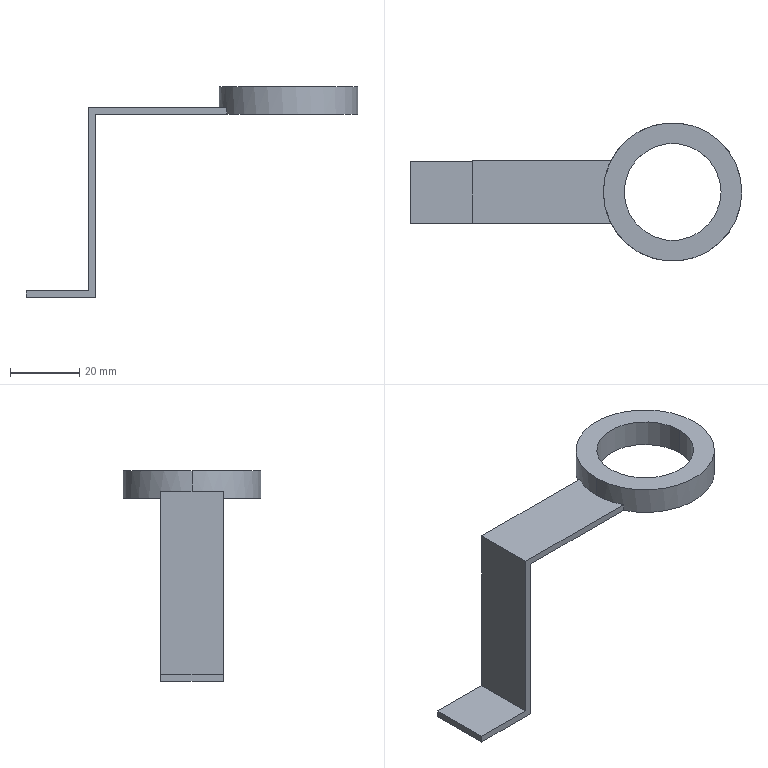Part | SolidWorks | features ICE 3, Extrusion 1 | 1 solid | 14 faces | box 95.861 x 40 x 61 mm | volume 9071 mm3 | plane 10 | cylinder 4 | commonest cylinder face diameters 28 x2 40 x2
STEP:
#1=CARTESIAN_POINT('',(-14.,0.,4.));
#2=VERTEX_POINT('',#1);
#3=CARTESIAN_POINT('',(14.,0.,4.));
#4=VERTEX_POINT('',#3);
#5=CARTESIAN_POINT('',(0.,0.,4.));
#6=DIRECTION('',(0.,0.,1.));
#7=DIRECTION('',(1.,0.,0.));
#8=AXIS2_PLACEMENT_3D('',#5,#6,#7);
#9=CIRCLE('',#8,14.);
#10=EDGE_CURVE('',#2,#4,#9,.T.);
#11=ORIENTED_EDGE('',*,*,#10,.T.);
#12=CARTESIAN_POINT('',(14.,0.,-4.));
#13=VERTEX_POINT('',#12);
#14=CARTESIAN_POINT('',(14.,0.,4.));
#15=DIRECTION('',(0.,0.,-1.));
#16=VECTOR('',#15,1000.);
#17=LINE('',#14,#16);
#18=EDGE_CURVE('',#4,#13,#17,.T.);
#19=ORIENTED_EDGE('',*,*,#18,.T.);
#20=CARTESIAN_POINT('',(-14.,0.,-4.));
#21=VERTEX_POINT('',#20);
#22=CARTESIAN_POINT('',(0.,0.,-4.));
#23=DIRECTION('',(0.,0.,1.));
#24=DIRECTION('',(1.,0.,0.));
#25=AXIS2_PLACEMENT_3D('',#22,#23,#24);
#26=CIRCLE('',#25,14.);
#27=EDGE_CURVE('',#21,#13,#26,.T.);
#28=ORIENTED_EDGE('',*,*,#27,.F.);
#29=CARTESIAN_POINT('',(-14.,0.,4.));
#30=DIRECTION('',(0.,0.,-1.));
#31=VECTOR('',#30,1000.);
#32=LINE('',#29,#31);
#33=EDGE_CURVE('',#2,#21,#32,.T.);
#34=ORIENTED_EDGE('',*,*,#33,.F.);
#35=EDGE_LOOP('',(#11,#19,#28,#34));
#36=FACE_OUTER_BOUND('',#35,.T.);
#37=CARTESIAN_POINT('',(0.,0.,4.));
#38=DIRECTION('',(0.,0.,-1.));
#39=DIRECTION('',(-1.,0.,0.));
#40=AXIS2_PLACEMENT_3D('',#37,#38,#39);
#41=CYLINDRICAL_SURFACE('',#40,14.);
#42=ADVANCED_FACE('',(#36),#41,.F.);
#43=CARTESIAN_POINT('',(20.,0.,4.));
#44=VERTEX_POINT('',#43);
#45=CARTESIAN_POINT('',(-20.,0.,4.));
#46=VERTEX_POINT('',#45);
#47=CARTESIAN_POINT('',(0.,0.,4.));
#48=DIRECTION('',(0.,0.,1.));
#49=DIRECTION('',(1.,0.,0.));
#50=AXIS2_PLACEMENT_3D('',#47,#48,#49);
#51=CIRCLE('',#50,20.);
#52=EDGE_CURVE('',#44,#46,#51,.T.);
#53=ORIENTED_EDGE('',*,*,#52,.F.);
#54=CARTESIAN_POINT('',(20.,0.,-4.));
#55=VERTEX_POINT('',#54);
#56=CARTESIAN_POINT('',(20.,0.,4.));
#57=DIRECTION('',(0.,0.,-1.));
#58=VECTOR('',#57,1000.);
#59=LINE('',#56,#58);
#60=EDGE_CURVE('',#44,#55,#59,.T.);
#61=ORIENTED_EDGE('',*,*,#60,.T.);
#62=CARTESIAN_POINT('',(-17.861,9.,-4.));
#63=VERTEX_POINT('',#62);
#64=CARTESIAN_POINT('',(0.,0.,-4.));
#65=DIRECTION('',(0.,0.,1.));
#66=DIRECTION('',(1.,0.,0.));
#67=AXIS2_PLACEMENT_3D('',#64,#65,#66);
#68=CIRCLE('',#67,20.);
#69=EDGE_CURVE('',#55,#63,#68,.T.);
#70=ORIENTED_EDGE('',*,*,#69,.T.);
#71=CARTESIAN_POINT('',(-17.861,9.,-2.));
#72=VERTEX_POINT('',#71);
#73=CARTESIAN_POINT('',(-17.861,9.,-2.));
#74=DIRECTION('',(0.,0.,-1.));
#75=VECTOR('',#74,1000.);
#76=LINE('',#73,#75);
#77=EDGE_CURVE('',#72,#63,#76,.T.);
#78=ORIENTED_EDGE('',*,*,#77,.F.);
#79=CARTESIAN_POINT('',(-20.,0.,-2.));
#80=VERTEX_POINT('',#79);
#81=CARTESIAN_POINT('',(0.,0.,-2.));
#82=DIRECTION('',(0.,0.,1.));
#83=DIRECTION('',(1.,0.,0.));
#84=AXIS2_PLACEMENT_3D('',#81,#82,#83);
#85=CIRCLE('',#84,20.);
#86=EDGE_CURVE('',#72,#80,#85,.T.);
#87=ORIENTED_EDGE('',*,*,#86,.T.);
#88=CARTESIAN_POINT('',(-20.,0.,4.));
#89=DIRECTION('',(0.,0.,-1.));
#90=VECTOR('',#89,1000.);
#91=LINE('',#88,#90);
#92=EDGE_CURVE('',#46,#80,#91,.T.);
#93=ORIENTED_EDGE('',*,*,#92,.F.);
#94=EDGE_LOOP('',(#53,#61,#70,#78,#87,#93));
#95=FACE_OUTER_BOUND('',#94,.T.);
#96=CARTESIAN_POINT('',(0.,0.,4.));
#97=DIRECTION('',(0.,0.,-1.));
#98=DIRECTION('',(-1.,0.,0.));
#99=AXIS2_PLACEMENT_3D('',#96,#97,#98);
#100=CYLINDRICAL_SURFACE('',#99,20.);
#101=ADVANCED_FACE('',(#95),#100,.T.);
#102=ORIENTED_EDGE('',*,*,#27,.T.);
#103=CARTESIAN_POINT('',(0.,0.,-4.));
#104=DIRECTION('',(0.,0.,1.));
#105=DIRECTION('',(1.,0.,0.));
#106=AXIS2_PLACEMENT_3D('',#103,#104,#105);
#107=CIRCLE('',#106,14.);
#108=EDGE_CURVE('',#13,#21,#107,.T.);
#109=ORIENTED_EDGE('',*,*,#108,.T.);
#110=EDGE_LOOP('',(#102,#109));
#111=FACE_BOUND('',#110,.T.);
#112=CARTESIAN_POINT('',(-55.861,9.,-4.));
#113=VERTEX_POINT('',#112);
#114=CARTESIAN_POINT('',(-55.861,-9.,-4.));
#115=VERTEX_POINT('',#114);
#116=CARTESIAN_POINT('',(-55.861,9.,-4.));
#117=DIRECTION('',(0.,-1.,0.));
#118=VECTOR('',#117,1000.);
#119=LINE('',#116,#118);
#120=EDGE_CURVE('',#113,#115,#119,.T.);
#121=ORIENTED_EDGE('',*,*,#120,.F.);
#122=CARTESIAN_POINT('',(-17.861,9.,-4.));
#123=DIRECTION('',(1.,0.,0.));
#124=VECTOR('',#123,1000.);
#125=LINE('',#122,#124);
#126=EDGE_CURVE('',#113,#63,#125,.T.);
#127=ORIENTED_EDGE('',*,*,#126,.T.);
#128=ORIENTED_EDGE('',*,*,#69,.F.);
#129=CARTESIAN_POINT('',(-17.861,-9.,-4.));
#130=VERTEX_POINT('',#129);
#131=CARTESIAN_POINT('',(0.,0.,-4.));
#132=DIRECTION('',(0.,0.,1.));
#133=DIRECTION('',(1.,0.,0.));
#134=AXIS2_PLACEMENT_3D('',#131,#132,#133);
#135=CIRCLE('',#134,20.);
#136=EDGE_CURVE('',#130,#55,#135,.T.);
#137=ORIENTED_EDGE('',*,*,#136,.F.);
#138=CARTESIAN_POINT('',(-57.861,-9.,-4.));
#139=DIRECTION('',(-1.,0.,0.));
#140=VECTOR('',#139,1000.);
#141=LINE('',#138,#140);
#142=EDGE_CURVE('',#130,#115,#141,.T.);
#143=ORIENTED_EDGE('',*,*,#142,.T.);
#144=EDGE_LOOP('',(#121,#127,#128,#137,#143));
#145=FACE_OUTER_BOUND('',#144,.T.);
#146=CARTESIAN_POINT('',(0.,0.,-4.));
#147=DIRECTION('',(0.,0.,1.));
#148=DIRECTION('',(1.,0.,0.));
#149=AXIS2_PLACEMENT_3D('',#146,#147,#148);
#150=PLANE('',#149);
#151=ADVANCED_FACE('',(#111,#145),#150,.F.);
#152=CARTESIAN_POINT('',(0.,0.,4.));
#153=DIRECTION('',(0.,0.,1.));
#154=DIRECTION('',(1.,0.,0.));
#155=AXIS2_PLACEMENT_3D('',#152,#153,#154);
#156=CIRCLE('',#155,20.);
#157=EDGE_CURVE('',#46,#44,#156,.T.);
#158=ORIENTED_EDGE('',*,*,#157,.T.);
#159=ORIENTED_EDGE('',*,*,#52,.T.);
#160=EDGE_LOOP('',(#158,#159));
#161=FACE_OUTER_BOUND('',#160,.T.);
#162=ORIENTED_EDGE('',*,*,#10,.F.);
#163=CARTESIAN_POINT('',(0.,0.,4.));
#164=DIRECTION('',(0.,0.,1.));
#165=DIRECTION('',(1.,0.,0.));
#166=AXIS2_PLACEMENT_3D('',#163,#164,#165);
#167=CIRCLE('',#166,14.);
#168=EDGE_CURVE('',#4,#2,#167,.T.);
#169=ORIENTED_EDGE('',*,*,#168,.F.);
#170=EDGE_LOOP('',(#162,#169));
#171=FACE_BOUND('',#170,.T.);
#172=CARTESIAN_POINT('',(0.,0.,4.));
#173=DIRECTION('',(0.,0.,1.));
#174=DIRECTION('',(1.,0.,0.));
#175=AXIS2_PLACEMENT_3D('',#172,#173,#174);
#176=PLANE('',#175);
#177=ADVANCED_FACE('',(#161,#171),#176,.T.);
#178=ORIENTED_EDGE('',*,*,#60,.F.);
#179=ORIENTED_EDGE('',*,*,#157,.F.);
#180=ORIENTED_EDGE('',*,*,#92,.T.);
#181=CARTESIAN_POINT('',(-17.861,-9.,-2.));
#182=VERTEX_POINT('',#181);
#183=CARTESIAN_POINT('',(0.,0.,-2.));
#184=DIRECTION('',(0.,0.,1.));
#185=DIRECTION('',(1.,0.,0.));
#186=AXIS2_PLACEMENT_3D('',#183,#184,#185);
#187=CIRCLE('',#186,20.);
#188=EDGE_CURVE('',#80,#182,#187,.T.);
#189=ORIENTED_EDGE('',*,*,#188,.T.);
#190=CARTESIAN_POINT('',(-17.861,-9.,-2.));
#191=DIRECTION('',(0.,0.,-1.));
#192=VECTOR('',#191,1000.);
#193=LINE('',#190,#192);
#194=EDGE_CURVE('',#182,#130,#193,.T.);
#195=ORIENTED_EDGE('',*,*,#194,.T.);
#196=ORIENTED_EDGE('',*,*,#136,.T.);
#197=EDGE_LOOP('',(#178,#179,#180,#189,#195,#196));
#198=FACE_OUTER_BOUND('',#197,.T.);
#199=CARTESIAN_POINT('',(0.,0.,4.));
#200=DIRECTION('',(0.,0.,-1.));
#201=DIRECTION('',(-1.,0.,0.));
#202=AXIS2_PLACEMENT_3D('',#199,#200,#201);
#203=CYLINDRICAL_SURFACE('',#202,20.);
#204=ADVANCED_FACE('',(#198),#203,.T.);
#205=ORIENTED_EDGE('',*,*,#18,.F.);
#206=ORIENTED_EDGE('',*,*,#168,.T.);
#207=ORIENTED_EDGE('',*,*,#33,.T.);
#208=ORIENTED_EDGE('',*,*,#108,.F.);
#209=EDGE_LOOP('',(#205,#206,#207,#208));
#210=FACE_OUTER_BOUND('',#209,.T.);
#211=CARTESIAN_POINT('',(0.,0.,4.));
#212=DIRECTION('',(0.,0.,-1.));
#213=DIRECTION('',(-1.,0.,0.));
#214=AXIS2_PLACEMENT_3D('',#211,#212,#213);
#215=CYLINDRICAL_SURFACE('',#214,14.);
#216=ADVANCED_FACE('',(#210),#215,.F.);
#217=ORIENTED_EDGE('',*,*,#126,.F.);
#218=CARTESIAN_POINT('',(-55.861,9.,-57.));
#219=VERTEX_POINT('',#218);
#220=CARTESIAN_POINT('',(-55.861,9.,-57.));
#221=DIRECTION('',(0.,0.,1.));
#222=VECTOR('',#221,1000.);
#223=LINE('',#220,#222);
#224=EDGE_CURVE('',#219,#113,#223,.T.);
#225=ORIENTED_EDGE('',*,*,#224,.F.);
#226=CARTESIAN_POINT('',(-75.861,9.,-57.));
#227=VERTEX_POINT('',#226);
#228=CARTESIAN_POINT('',(-57.861,9.,-57.));
#229=DIRECTION('',(1.,0.,0.));
#230=VECTOR('',#229,1000.);
#231=LINE('',#228,#230);
#232=EDGE_CURVE('',#227,#219,#231,.T.);
#233=ORIENTED_EDGE('',*,*,#232,.F.);
#234=CARTESIAN_POINT('',(-75.861,9.,-55.));
#235=VERTEX_POINT('',#234);
#236=CARTESIAN_POINT('',(-75.861,9.,-57.));
#237=DIRECTION('',(0.,0.,-1.));
#238=VECTOR('',#237,1000.);
#239=LINE('',#236,#238);
#240=EDGE_CURVE('',#235,#227,#239,.T.);
#241=ORIENTED_EDGE('',*,*,#240,.F.);
#242=CARTESIAN_POINT('',(-57.861,9.,-55.));
#243=VERTEX_POINT('',#242);
#244=CARTESIAN_POINT('',(-75.861,9.,-55.));
#245=DIRECTION('',(1.,0.,0.));
#246=VECTOR('',#245,1000.);
#247=LINE('',#244,#246);
#248=EDGE_CURVE('',#235,#243,#247,.T.);
#249=ORIENTED_EDGE('',*,*,#248,.T.);
#250=CARTESIAN_POINT('',(-57.861,9.,-2.));
#251=VERTEX_POINT('',#250);
#252=CARTESIAN_POINT('',(-57.861,9.,-2.));
#253=DIRECTION('',(0.,0.,-1.));
#254=VECTOR('',#253,1000.);
#255=LINE('',#252,#254);
#256=EDGE_CURVE('',#251,#243,#255,.T.);
#257=ORIENTED_EDGE('',*,*,#256,.F.);
#258=CARTESIAN_POINT('',(-17.861,9.,-2.));
#259=DIRECTION('',(1.,0.,0.));
#260=VECTOR('',#259,1000.);
#261=LINE('',#258,#260);
#262=EDGE_CURVE('',#251,#72,#261,.T.);
#263=ORIENTED_EDGE('',*,*,#262,.T.);
#264=ORIENTED_EDGE('',*,*,#77,.T.);
#265=EDGE_LOOP('',(#217,#225,#233,#241,#249,#257,#263,#264));
#266=FACE_OUTER_BOUND('',#265,.T.);
#267=CARTESIAN_POINT('',(-17.861,9.,-2.));
#268=DIRECTION('',(0.,1.,0.));
#269=DIRECTION('',(0.,0.,1.));
#270=AXIS2_PLACEMENT_3D('',#267,#268,#269);
#271=PLANE('',#270);
#272=ADVANCED_FACE('',(#266),#271,.T.);
#273=CARTESIAN_POINT('',(-57.861,-9.,-55.));
#274=VERTEX_POINT('',#273);
#275=CARTESIAN_POINT('',(-57.861,9.,-55.));
#276=DIRECTION('',(0.,1.,0.));
#277=VECTOR('',#276,1000.);
#278=LINE('',#275,#277);
#279=EDGE_CURVE('',#274,#243,#278,.T.);
#280=ORIENTED_EDGE('',*,*,#279,.F.);
#281=CARTESIAN_POINT('',(-57.861,-9.,-2.));
#282=VERTEX_POINT('',#281);
#283=CARTESIAN_POINT('',(-57.861,-9.,-2.));
#284=DIRECTION('',(0.,0.,-1.));
#285=VECTOR('',#284,1000.);
#286=LINE('',#283,#285);
#287=EDGE_CURVE('',#282,#274,#286,.T.);
#288=ORIENTED_EDGE('',*,*,#287,.F.);
#289=CARTESIAN_POINT('',(-57.861,9.,-2.));
#290=DIRECTION('',(0.,1.,0.));
#291=VECTOR('',#290,1000.);
#292=LINE('',#289,#291);
#293=EDGE_CURVE('',#282,#251,#292,.T.);
#294=ORIENTED_EDGE('',*,*,#293,.T.);
#295=ORIENTED_EDGE('',*,*,#256,.T.);
#296=EDGE_LOOP('',(#280,#288,#294,#295));
#297=FACE_OUTER_BOUND('',#296,.T.);
#298=CARTESIAN_POINT('',(-57.861,9.,-2.));
#299=DIRECTION('',(-1.,0.,0.));
#300=DIRECTION('',(0.,0.,1.));
#301=AXIS2_PLACEMENT_3D('',#298,#299,#300);
#302=PLANE('',#301);
#303=ADVANCED_FACE('',(#297),#302,.T.);
#304=ORIENTED_EDGE('',*,*,#142,.F.);
#305=ORIENTED_EDGE('',*,*,#194,.F.);
#306=CARTESIAN_POINT('',(-57.861,-9.,-2.));
#307=DIRECTION('',(-1.,0.,0.));
#308=VECTOR('',#307,1000.);
#309=LINE('',#306,#308);
#310=EDGE_CURVE('',#182,#282,#309,.T.);
#311=ORIENTED_EDGE('',*,*,#310,.T.);
#312=ORIENTED_EDGE('',*,*,#287,.T.);
#313=CARTESIAN_POINT('',(-75.861,-9.,-55.));
#314=VERTEX_POINT('',#313);
#315=CARTESIAN_POINT('',(-75.861,-9.,-55.));
#316=DIRECTION('',(1.,0.,0.));
#317=VECTOR('',#316,1000.);
#318=LINE('',#315,#317);
#319=EDGE_CURVE('',#314,#274,#318,.T.);
#320=ORIENTED_EDGE('',*,*,#319,.F.);
#321=CARTESIAN_POINT('',(-75.861,-9.,-57.));
#322=VERTEX_POINT('',#321);
#323=CARTESIAN_POINT('',(-75.861,-9.,-57.));
#324=DIRECTION('',(0.,0.,1.));
#325=VECTOR('',#324,1000.);
#326=LINE('',#323,#325);
#327=EDGE_CURVE('',#322,#314,#326,.T.);
#328=ORIENTED_EDGE('',*,*,#327,.F.);
#329=CARTESIAN_POINT('',(-55.861,-9.,-57.));
#330=VERTEX_POINT('',#329);
#331=CARTESIAN_POINT('',(-57.861,-9.,-57.));
#332=DIRECTION('',(-1.,0.,0.));
#333=VECTOR('',#332,1000.);
#334=LINE('',#331,#333);
#335=EDGE_CURVE('',#330,#322,#334,.T.);
#336=ORIENTED_EDGE('',*,*,#335,.F.);
#337=CARTESIAN_POINT('',(-55.861,-9.,-57.));
#338=DIRECTION('',(0.,0.,1.));
#339=VECTOR('',#338,1000.);
#340=LINE('',#337,#339);
#341=EDGE_CURVE('',#330,#115,#340,.T.);
#342=ORIENTED_EDGE('',*,*,#341,.T.);
#343=EDGE_LOOP('',(#304,#305,#311,#312,#320,#328,#336,#342));
#344=FACE_OUTER_BOUND('',#343,.T.);
#345=CARTESIAN_POINT('',(-57.861,-9.,-2.));
#346=DIRECTION('',(0.,-1.,0.));
#347=DIRECTION('',(0.,0.,-1.));
#348=AXIS2_PLACEMENT_3D('',#345,#346,#347);
#349=PLANE('',#348);
#350=ADVANCED_FACE('',(#344),#349,.T.);
#351=ORIENTED_EDGE('',*,*,#86,.F.);
#352=ORIENTED_EDGE('',*,*,#262,.F.);
#353=ORIENTED_EDGE('',*,*,#293,.F.);
#354=ORIENTED_EDGE('',*,*,#310,.F.);
#355=ORIENTED_EDGE('',*,*,#188,.F.);
#356=EDGE_LOOP('',(#351,#352,#353,#354,#355));
#357=FACE_OUTER_BOUND('',#356,.T.);
#358=CARTESIAN_POINT('',(0.,0.,-2.));
#359=DIRECTION('',(0.,0.,1.));
#360=DIRECTION('',(1.,0.,0.));
#361=AXIS2_PLACEMENT_3D('',#358,#359,#360);
#362=PLANE('',#361);
#363=ADVANCED_FACE('',(#357),#362,.T.);
#364=ORIENTED_EDGE('',*,*,#120,.T.);
#365=ORIENTED_EDGE('',*,*,#341,.F.);
#366=CARTESIAN_POINT('',(-55.861,9.,-57.));
#367=DIRECTION('',(0.,-1.,0.));
#368=VECTOR('',#367,1000.);
#369=LINE('',#366,#368);
#370=EDGE_CURVE('',#219,#330,#369,.T.);
#371=ORIENTED_EDGE('',*,*,#370,.F.);
#372=ORIENTED_EDGE('',*,*,#224,.T.);
#373=EDGE_LOOP('',(#364,#365,#371,#372));
#374=FACE_OUTER_BOUND('',#373,.T.);
#375=CARTESIAN_POINT('',(-55.861,9.,-57.));
#376=DIRECTION('',(-1.,0.,0.));
#377=DIRECTION('',(0.,0.,1.));
#378=AXIS2_PLACEMENT_3D('',#375,#376,#377);
#379=PLANE('',#378);
#380=ADVANCED_FACE('',(#374),#379,.F.);
#381=ORIENTED_EDGE('',*,*,#335,.T.);
#382=CARTESIAN_POINT('',(-75.861,9.,-57.));
#383=DIRECTION('',(0.,-1.,0.));
#384=VECTOR('',#383,1000.);
#385=LINE('',#382,#384);
#386=EDGE_CURVE('',#227,#322,#385,.T.);
#387=ORIENTED_EDGE('',*,*,#386,.F.);
#388=ORIENTED_EDGE('',*,*,#232,.T.);
#389=ORIENTED_EDGE('',*,*,#370,.T.);
#390=EDGE_LOOP('',(#381,#387,#388,#389));
#391=FACE_OUTER_BOUND('',#390,.T.);
#392=CARTESIAN_POINT('',(0.,0.,-57.));
#393=DIRECTION('',(0.,0.,1.));
#394=DIRECTION('',(1.,0.,0.));
#395=AXIS2_PLACEMENT_3D('',#392,#393,#394);
#396=PLANE('',#395);
#397=ADVANCED_FACE('',(#391),#396,.F.);
#398=ORIENTED_EDGE('',*,*,#279,.T.);
#399=ORIENTED_EDGE('',*,*,#248,.F.);
#400=CARTESIAN_POINT('',(-75.861,9.,-55.));
#401=DIRECTION('',(0.,1.,0.));
#402=VECTOR('',#401,1000.);
#403=LINE('',#400,#402);
#404=EDGE_CURVE('',#314,#235,#403,.T.);
#405=ORIENTED_EDGE('',*,*,#404,.F.);
#406=ORIENTED_EDGE('',*,*,#319,.T.);
#407=EDGE_LOOP('',(#398,#399,#405,#406));
#408=FACE_OUTER_BOUND('',#407,.T.);
#409=CARTESIAN_POINT('',(-75.861,9.,-55.));
#410=DIRECTION('',(0.,0.,-1.));
#411=DIRECTION('',(-1.,0.,0.));
#412=AXIS2_PLACEMENT_3D('',#409,#410,#411);
#413=PLANE('',#412);
#414=ADVANCED_FACE('',(#408),#413,.F.);
#415=ORIENTED_EDGE('',*,*,#386,.T.);
#416=ORIENTED_EDGE('',*,*,#327,.T.);
#417=ORIENTED_EDGE('',*,*,#404,.T.);
#418=ORIENTED_EDGE('',*,*,#240,.T.);
#419=EDGE_LOOP('',(#415,#416,#417,#418));
#420=FACE_OUTER_BOUND('',#419,.T.);
#421=CARTESIAN_POINT('',(-75.861,0.,0.));
#422=DIRECTION('',(-1.,0.,0.));
#423=DIRECTION('',(0.,0.,1.));
#424=AXIS2_PLACEMENT_3D('',#421,#422,#423);
#425=PLANE('',#424);
#426=ADVANCED_FACE('',(#420),#425,.T.);
#427=CLOSED_SHELL('',(#42,#101,#151,#177,#204,#216,#272,#303,#350,#363,#380,#397,#414,#426));
#428=MANIFOLD_SOLID_BREP('',#427);
#429=CARTESIAN_POINT('',(0.,0.,0.));
#430=DIRECTION('',(0.,0.,1.));
#431=DIRECTION('',(1.,0.,0.));
#432=AXIS2_PLACEMENT_3D('',#429,#430,#431);
#433=(LENGTH_UNIT()NAMED_UNIT(*)SI_UNIT(.MILLI.,.METRE.));
#434=UNCERTAINTY_MEASURE_WITH_UNIT(LENGTH_MEASURE(0.00001),#433,'','');
#435=(NAMED_UNIT(*)PLANE_ANGLE_UNIT()SI_UNIT($,.RADIAN.));
#436=(NAMED_UNIT(*)SI_UNIT($,.STERADIAN.)SOLID_ANGLE_UNIT());
#437=(GEOMETRIC_REPRESENTATION_CONTEXT(3)GLOBAL_UNCERTAINTY_ASSIGNED_CONTEXT((#434))GLOBAL_UNIT_ASSIGNED_CONTEXT((#433,#435,#436))REPRESENTATION_CONTEXT('',''));
#438=ADVANCED_BREP_SHAPE_REPRESENTATION('',(#428,#432),#437);